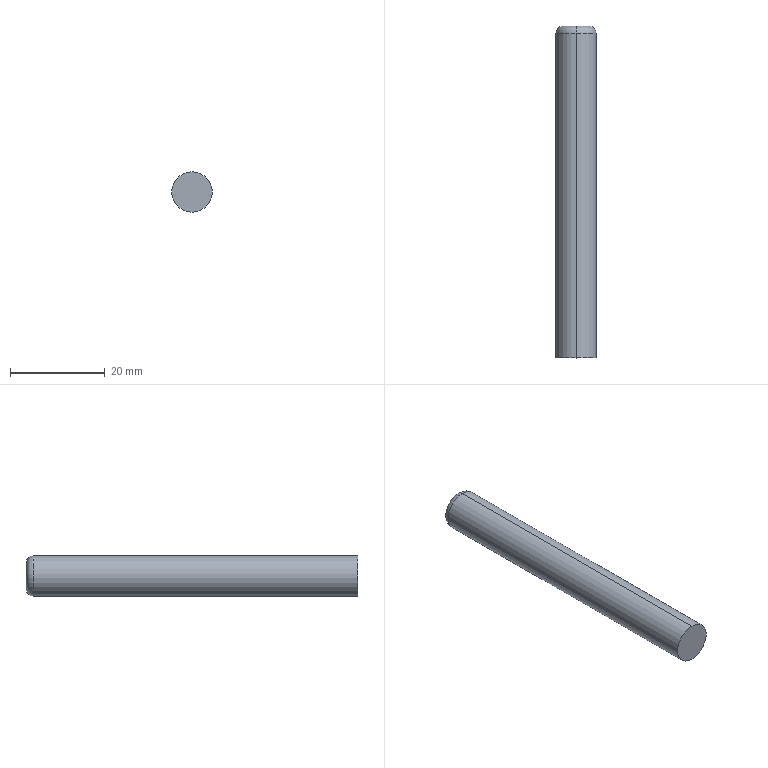Part | SolidWorks | features Extrusion 1, Fillet 1 | 1 solid | 6 faces | box 8.5 x 70 x 8.5 mm | volume 3960 mm3 | torus 2 | cylinder 2 | plane 2 | commonest cylinder face diameters 8.5 x2
STEP:
#1=CARTESIAN_POINT('',(0.,68.5,-4.25));
#2=VERTEX_POINT('',#1);
#3=CARTESIAN_POINT('',(0.,68.5,4.25));
#4=VERTEX_POINT('',#3);
#5=CARTESIAN_POINT('',(0.,68.5,0.));
#6=DIRECTION('',(0.,-1.,0.));
#7=DIRECTION('',(0.,0.,1.));
#8=AXIS2_PLACEMENT_3D('',#5,#6,#7);
#9=CIRCLE('',#8,4.25);
#10=EDGE_CURVE('',#2,#4,#9,.T.);
#11=ORIENTED_EDGE('',*,*,#10,.F.);
#12=CARTESIAN_POINT('',(0.,70.,-2.75));
#13=VERTEX_POINT('',#12);
#14=CARTESIAN_POINT('',(0.,68.5,-2.75));
#15=DIRECTION('',(1.,0.,0.));
#16=DIRECTION('',(0.,0.,-1.));
#17=AXIS2_PLACEMENT_3D('',#14,#15,#16);
#18=CIRCLE('',#17,1.5);
#19=EDGE_CURVE('',#2,#13,#18,.T.);
#20=ORIENTED_EDGE('',*,*,#19,.T.);
#21=CARTESIAN_POINT('',(0.,70.,2.75));
#22=VERTEX_POINT('',#21);
#23=CARTESIAN_POINT('',(0.,70.,0.));
#24=DIRECTION('',(0.,1.,0.));
#25=DIRECTION('',(0.,0.,1.));
#26=AXIS2_PLACEMENT_3D('',#23,#24,#25);
#27=CIRCLE('',#26,2.75);
#28=EDGE_CURVE('',#22,#13,#27,.T.);
#29=ORIENTED_EDGE('',*,*,#28,.F.);
#30=CARTESIAN_POINT('',(0.,68.5,2.75));
#31=DIRECTION('',(-1.,0.,0.));
#32=DIRECTION('',(0.,0.,1.));
#33=AXIS2_PLACEMENT_3D('',#30,#31,#32);
#34=CIRCLE('',#33,1.5);
#35=EDGE_CURVE('',#4,#22,#34,.T.);
#36=ORIENTED_EDGE('',*,*,#35,.F.);
#37=EDGE_LOOP('',(#11,#20,#29,#36));
#38=FACE_OUTER_BOUND('',#37,.T.);
#39=CARTESIAN_POINT('',(0.,68.5,0.));
#40=DIRECTION('',(0.,1.,0.));
#41=DIRECTION('',(0.,0.,1.));
#42=AXIS2_PLACEMENT_3D('',#39,#40,#41);
#43=TOROIDAL_SURFACE('',#42,2.75,1.5);
#44=ADVANCED_FACE('',(#38),#43,.T.);
#45=ORIENTED_EDGE('',*,*,#10,.T.);
#46=CARTESIAN_POINT('',(0.,0.,4.25));
#47=VERTEX_POINT('',#46);
#48=CARTESIAN_POINT('',(0.,70.,4.25));
#49=DIRECTION('',(0.,-1.,0.));
#50=VECTOR('',#49,1000.);
#51=LINE('',#48,#50);
#52=EDGE_CURVE('',#4,#47,#51,.T.);
#53=ORIENTED_EDGE('',*,*,#52,.T.);
#54=CARTESIAN_POINT('',(0.,0.,-4.25));
#55=VERTEX_POINT('',#54);
#56=CARTESIAN_POINT('',(0.,0.,0.));
#57=DIRECTION('',(0.,1.,0.));
#58=DIRECTION('',(0.,0.,1.));
#59=AXIS2_PLACEMENT_3D('',#56,#57,#58);
#60=CIRCLE('',#59,4.25);
#61=EDGE_CURVE('',#47,#55,#60,.T.);
#62=ORIENTED_EDGE('',*,*,#61,.T.);
#63=CARTESIAN_POINT('',(0.,70.,-4.25));
#64=DIRECTION('',(0.,-1.,0.));
#65=VECTOR('',#64,1000.);
#66=LINE('',#63,#65);
#67=EDGE_CURVE('',#2,#55,#66,.T.);
#68=ORIENTED_EDGE('',*,*,#67,.F.);
#69=EDGE_LOOP('',(#45,#53,#62,#68));
#70=FACE_OUTER_BOUND('',#69,.T.);
#71=CARTESIAN_POINT('',(0.,70.,0.));
#72=DIRECTION('',(0.,-1.,0.));
#73=DIRECTION('',(0.,0.,-1.));
#74=AXIS2_PLACEMENT_3D('',#71,#72,#73);
#75=CYLINDRICAL_SURFACE('',#74,4.25);
#76=ADVANCED_FACE('',(#70),#75,.T.);
#77=ORIENTED_EDGE('',*,*,#52,.F.);
#78=CARTESIAN_POINT('',(0.,68.5,0.));
#79=DIRECTION('',(0.,-1.,0.));
#80=DIRECTION('',(0.,0.,1.));
#81=AXIS2_PLACEMENT_3D('',#78,#79,#80);
#82=CIRCLE('',#81,4.25);
#83=EDGE_CURVE('',#4,#2,#82,.T.);
#84=ORIENTED_EDGE('',*,*,#83,.T.);
#85=ORIENTED_EDGE('',*,*,#67,.T.);
#86=CARTESIAN_POINT('',(0.,0.,0.));
#87=DIRECTION('',(0.,1.,0.));
#88=DIRECTION('',(0.,0.,1.));
#89=AXIS2_PLACEMENT_3D('',#86,#87,#88);
#90=CIRCLE('',#89,4.25);
#91=EDGE_CURVE('',#55,#47,#90,.T.);
#92=ORIENTED_EDGE('',*,*,#91,.T.);
#93=EDGE_LOOP('',(#77,#84,#85,#92));
#94=FACE_OUTER_BOUND('',#93,.T.);
#95=CARTESIAN_POINT('',(0.,70.,0.));
#96=DIRECTION('',(0.,-1.,0.));
#97=DIRECTION('',(0.,0.,-1.));
#98=AXIS2_PLACEMENT_3D('',#95,#96,#97);
#99=CYLINDRICAL_SURFACE('',#98,4.25);
#100=ADVANCED_FACE('',(#94),#99,.T.);
#101=ORIENTED_EDGE('',*,*,#28,.T.);
#102=CARTESIAN_POINT('',(0.,70.,0.));
#103=DIRECTION('',(0.,1.,0.));
#104=DIRECTION('',(0.,0.,1.));
#105=AXIS2_PLACEMENT_3D('',#102,#103,#104);
#106=CIRCLE('',#105,2.75);
#107=EDGE_CURVE('',#13,#22,#106,.T.);
#108=ORIENTED_EDGE('',*,*,#107,.T.);
#109=EDGE_LOOP('',(#101,#108));
#110=FACE_OUTER_BOUND('',#109,.T.);
#111=CARTESIAN_POINT('',(0.,70.,0.));
#112=DIRECTION('',(0.,1.,0.));
#113=DIRECTION('',(0.,0.,1.));
#114=AXIS2_PLACEMENT_3D('',#111,#112,#113);
#115=PLANE('',#114);
#116=ADVANCED_FACE('',(#110),#115,.T.);
#117=ORIENTED_EDGE('',*,*,#91,.F.);
#118=ORIENTED_EDGE('',*,*,#61,.F.);
#119=EDGE_LOOP('',(#117,#118));
#120=FACE_OUTER_BOUND('',#119,.T.);
#121=CARTESIAN_POINT('',(0.,0.,0.));
#122=DIRECTION('',(0.,1.,0.));
#123=DIRECTION('',(0.,0.,1.));
#124=AXIS2_PLACEMENT_3D('',#121,#122,#123);
#125=PLANE('',#124);
#126=ADVANCED_FACE('',(#120),#125,.F.);
#127=ORIENTED_EDGE('',*,*,#19,.F.);
#128=ORIENTED_EDGE('',*,*,#83,.F.);
#129=ORIENTED_EDGE('',*,*,#35,.T.);
#130=ORIENTED_EDGE('',*,*,#107,.F.);
#131=EDGE_LOOP('',(#127,#128,#129,#130));
#132=FACE_OUTER_BOUND('',#131,.T.);
#133=CARTESIAN_POINT('',(0.,68.5,0.));
#134=DIRECTION('',(0.,1.,0.));
#135=DIRECTION('',(0.,0.,1.));
#136=AXIS2_PLACEMENT_3D('',#133,#134,#135);
#137=TOROIDAL_SURFACE('',#136,2.75,1.5);
#138=ADVANCED_FACE('',(#132),#137,.T.);
#139=CLOSED_SHELL('',(#44,#76,#100,#116,#126,#138));
#140=MANIFOLD_SOLID_BREP('',#139);
#141=CARTESIAN_POINT('',(0.,0.,0.));
#142=DIRECTION('',(0.,0.,1.));
#143=DIRECTION('',(1.,0.,0.));
#144=AXIS2_PLACEMENT_3D('',#141,#142,#143);
#145=(LENGTH_UNIT()NAMED_UNIT(*)SI_UNIT(.MILLI.,.METRE.));
#146=UNCERTAINTY_MEASURE_WITH_UNIT(LENGTH_MEASURE(0.00001),#145,'','');
#147=(NAMED_UNIT(*)PLANE_ANGLE_UNIT()SI_UNIT($,.RADIAN.));
#148=(NAMED_UNIT(*)SI_UNIT($,.STERADIAN.)SOLID_ANGLE_UNIT());
#149=(GEOMETRIC_REPRESENTATION_CONTEXT(3)GLOBAL_UNCERTAINTY_ASSIGNED_CONTEXT((#146))GLOBAL_UNIT_ASSIGNED_CONTEXT((#145,#147,#148))REPRESENTATION_CONTEXT('',''));
#150=ADVANCED_BREP_SHAPE_REPRESENTATION('',(#140,#144),#149);